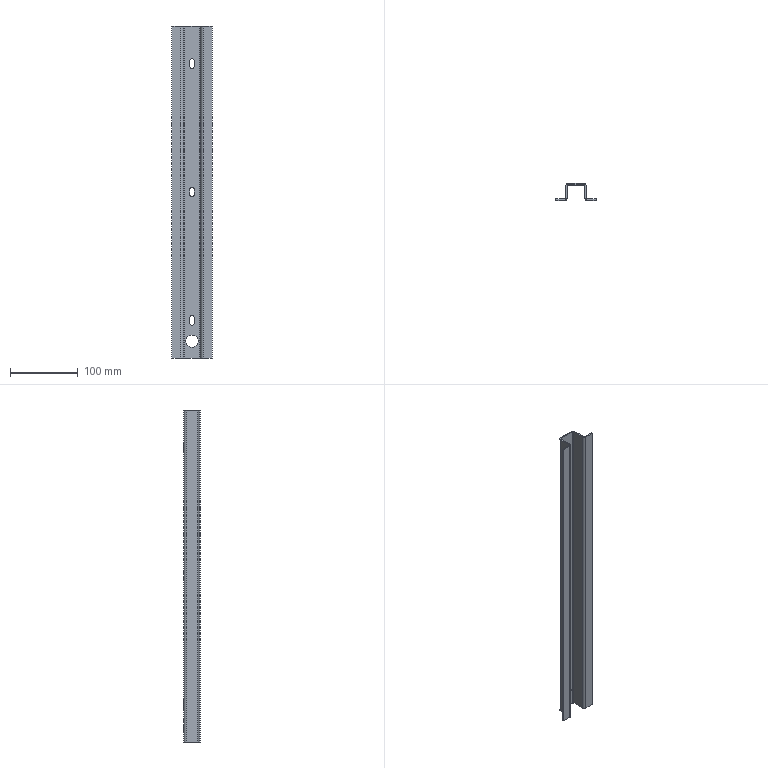Part | STEP file | SYL_0392D6J1SYL0380DJ100-657039 | 1 solid | 58 faces | box 60 x 25 x 491 mm | volume 98000 mm3 | plane 36 | cylinder 22 | commonest cylinder face diameters 7 x12 4 x4 8 x4 18 x2